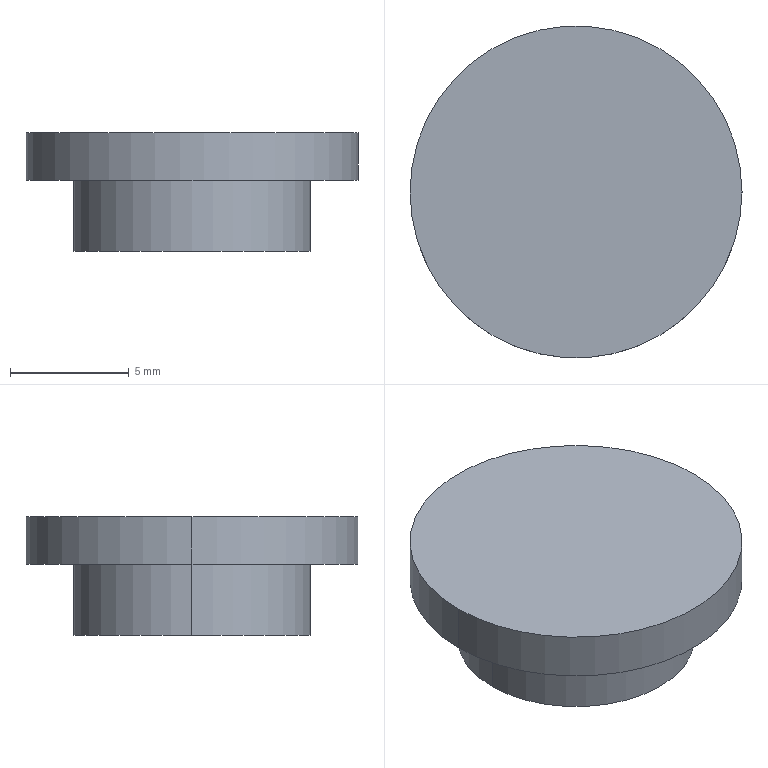Part | SolidWorks | features Extrusion 1, ICE 1 | 1 solid | 7 faces | box 14 x 14 x 5 mm | volume 543.496 mm3 | cylinder 4 | plane 3 | commonest cylinder face diameters 10 x2 14 x2
STEP:
#1=CARTESIAN_POINT('',(7.,0.,2.));
#2=VERTEX_POINT('',#1);
#3=CARTESIAN_POINT('',(-7.,0.,2.));
#4=VERTEX_POINT('',#3);
#5=CARTESIAN_POINT('',(0.,0.,2.));
#6=DIRECTION('',(0.,0.,1.));
#7=DIRECTION('',(1.,0.,0.));
#8=AXIS2_PLACEMENT_3D('',#5,#6,#7);
#9=CIRCLE('',#8,7.);
#10=EDGE_CURVE('',#2,#4,#9,.T.);
#11=ORIENTED_EDGE('',*,*,#10,.F.);
#12=CARTESIAN_POINT('',(7.,0.,0.));
#13=VERTEX_POINT('',#12);
#14=CARTESIAN_POINT('',(7.,0.,2.));
#15=DIRECTION('',(0.,0.,-1.));
#16=VECTOR('',#15,1000.);
#17=LINE('',#14,#16);
#18=EDGE_CURVE('',#2,#13,#17,.T.);
#19=ORIENTED_EDGE('',*,*,#18,.T.);
#20=CARTESIAN_POINT('',(-7.,0.,0.));
#21=VERTEX_POINT('',#20);
#22=CARTESIAN_POINT('',(0.,0.,0.));
#23=DIRECTION('',(0.,0.,1.));
#24=DIRECTION('',(1.,0.,0.));
#25=AXIS2_PLACEMENT_3D('',#22,#23,#24);
#26=CIRCLE('',#25,7.);
#27=EDGE_CURVE('',#13,#21,#26,.T.);
#28=ORIENTED_EDGE('',*,*,#27,.T.);
#29=CARTESIAN_POINT('',(-7.,0.,2.));
#30=DIRECTION('',(0.,0.,-1.));
#31=VECTOR('',#30,1000.);
#32=LINE('',#29,#31);
#33=EDGE_CURVE('',#4,#21,#32,.T.);
#34=ORIENTED_EDGE('',*,*,#33,.F.);
#35=EDGE_LOOP('',(#11,#19,#28,#34));
#36=FACE_OUTER_BOUND('',#35,.T.);
#37=CARTESIAN_POINT('',(0.,0.,2.));
#38=DIRECTION('',(0.,0.,-1.));
#39=DIRECTION('',(-1.,0.,0.));
#40=AXIS2_PLACEMENT_3D('',#37,#38,#39);
#41=CYLINDRICAL_SURFACE('',#40,7.);
#42=ADVANCED_FACE('',(#36),#41,.T.);
#43=CARTESIAN_POINT('',(5.,0.,-3.));
#44=VERTEX_POINT('',#43);
#45=CARTESIAN_POINT('',(-5.,0.,-3.));
#46=VERTEX_POINT('',#45);
#47=CARTESIAN_POINT('',(0.,0.,-3.));
#48=DIRECTION('',(0.,0.,1.));
#49=DIRECTION('',(1.,0.,0.));
#50=AXIS2_PLACEMENT_3D('',#47,#48,#49);
#51=CIRCLE('',#50,5.);
#52=EDGE_CURVE('',#44,#46,#51,.T.);
#53=ORIENTED_EDGE('',*,*,#52,.T.);
#54=CARTESIAN_POINT('',(-5.,0.,0.));
#55=VERTEX_POINT('',#54);
#56=CARTESIAN_POINT('',(-5.,0.,-3.));
#57=DIRECTION('',(0.,0.,1.));
#58=VECTOR('',#57,1000.);
#59=LINE('',#56,#58);
#60=EDGE_CURVE('',#46,#55,#59,.T.);
#61=ORIENTED_EDGE('',*,*,#60,.T.);
#62=CARTESIAN_POINT('',(5.,0.,0.));
#63=VERTEX_POINT('',#62);
#64=CARTESIAN_POINT('',(0.,0.,0.));
#65=DIRECTION('',(0.,0.,1.));
#66=DIRECTION('',(1.,0.,0.));
#67=AXIS2_PLACEMENT_3D('',#64,#65,#66);
#68=CIRCLE('',#67,5.);
#69=EDGE_CURVE('',#63,#55,#68,.T.);
#70=ORIENTED_EDGE('',*,*,#69,.F.);
#71=CARTESIAN_POINT('',(5.,0.,-3.));
#72=DIRECTION('',(0.,0.,1.));
#73=VECTOR('',#72,1000.);
#74=LINE('',#71,#73);
#75=EDGE_CURVE('',#44,#63,#74,.T.);
#76=ORIENTED_EDGE('',*,*,#75,.F.);
#77=EDGE_LOOP('',(#53,#61,#70,#76));
#78=FACE_OUTER_BOUND('',#77,.T.);
#79=CARTESIAN_POINT('',(0.,0.,-3.));
#80=DIRECTION('',(0.,0.,1.));
#81=DIRECTION('',(1.,0.,0.));
#82=AXIS2_PLACEMENT_3D('',#79,#80,#81);
#83=CYLINDRICAL_SURFACE('',#82,5.);
#84=ADVANCED_FACE('',(#78),#83,.T.);
#85=ORIENTED_EDGE('',*,*,#60,.F.);
#86=CARTESIAN_POINT('',(0.,0.,-3.));
#87=DIRECTION('',(0.,0.,1.));
#88=DIRECTION('',(1.,0.,0.));
#89=AXIS2_PLACEMENT_3D('',#86,#87,#88);
#90=CIRCLE('',#89,5.);
#91=EDGE_CURVE('',#46,#44,#90,.T.);
#92=ORIENTED_EDGE('',*,*,#91,.T.);
#93=ORIENTED_EDGE('',*,*,#75,.T.);
#94=CARTESIAN_POINT('',(0.,0.,0.));
#95=DIRECTION('',(0.,0.,1.));
#96=DIRECTION('',(1.,0.,0.));
#97=AXIS2_PLACEMENT_3D('',#94,#95,#96);
#98=CIRCLE('',#97,5.);
#99=EDGE_CURVE('',#55,#63,#98,.T.);
#100=ORIENTED_EDGE('',*,*,#99,.F.);
#101=EDGE_LOOP('',(#85,#92,#93,#100));
#102=FACE_OUTER_BOUND('',#101,.T.);
#103=CARTESIAN_POINT('',(0.,0.,-3.));
#104=DIRECTION('',(0.,0.,1.));
#105=DIRECTION('',(1.,0.,0.));
#106=AXIS2_PLACEMENT_3D('',#103,#104,#105);
#107=CYLINDRICAL_SURFACE('',#106,5.);
#108=ADVANCED_FACE('',(#102),#107,.T.);
#109=ORIENTED_EDGE('',*,*,#52,.F.);
#110=ORIENTED_EDGE('',*,*,#91,.F.);
#111=EDGE_LOOP('',(#109,#110));
#112=FACE_OUTER_BOUND('',#111,.T.);
#113=CARTESIAN_POINT('',(0.,0.,-3.));
#114=DIRECTION('',(0.,0.,1.));
#115=DIRECTION('',(1.,0.,0.));
#116=AXIS2_PLACEMENT_3D('',#113,#114,#115);
#117=PLANE('',#116);
#118=ADVANCED_FACE('',(#112),#117,.F.);
#119=ORIENTED_EDGE('',*,*,#18,.F.);
#120=CARTESIAN_POINT('',(0.,0.,2.));
#121=DIRECTION('',(0.,0.,1.));
#122=DIRECTION('',(1.,0.,0.));
#123=AXIS2_PLACEMENT_3D('',#120,#121,#122);
#124=CIRCLE('',#123,7.);
#125=EDGE_CURVE('',#4,#2,#124,.T.);
#126=ORIENTED_EDGE('',*,*,#125,.F.);
#127=ORIENTED_EDGE('',*,*,#33,.T.);
#128=CARTESIAN_POINT('',(0.,0.,0.));
#129=DIRECTION('',(0.,0.,1.));
#130=DIRECTION('',(1.,0.,0.));
#131=AXIS2_PLACEMENT_3D('',#128,#129,#130);
#132=CIRCLE('',#131,7.);
#133=EDGE_CURVE('',#21,#13,#132,.T.);
#134=ORIENTED_EDGE('',*,*,#133,.T.);
#135=EDGE_LOOP('',(#119,#126,#127,#134));
#136=FACE_OUTER_BOUND('',#135,.T.);
#137=CARTESIAN_POINT('',(0.,0.,2.));
#138=DIRECTION('',(0.,0.,-1.));
#139=DIRECTION('',(-1.,0.,0.));
#140=AXIS2_PLACEMENT_3D('',#137,#138,#139);
#141=CYLINDRICAL_SURFACE('',#140,7.);
#142=ADVANCED_FACE('',(#136),#141,.T.);
#143=ORIENTED_EDGE('',*,*,#125,.T.);
#144=ORIENTED_EDGE('',*,*,#10,.T.);
#145=EDGE_LOOP('',(#143,#144));
#146=FACE_OUTER_BOUND('',#145,.T.);
#147=CARTESIAN_POINT('',(0.,0.,2.));
#148=DIRECTION('',(0.,0.,1.));
#149=DIRECTION('',(1.,0.,0.));
#150=AXIS2_PLACEMENT_3D('',#147,#148,#149);
#151=PLANE('',#150);
#152=ADVANCED_FACE('',(#146),#151,.T.);
#153=ORIENTED_EDGE('',*,*,#69,.T.);
#154=ORIENTED_EDGE('',*,*,#99,.T.);
#155=EDGE_LOOP('',(#153,#154));
#156=FACE_BOUND('',#155,.T.);
#157=ORIENTED_EDGE('',*,*,#133,.F.);
#158=ORIENTED_EDGE('',*,*,#27,.F.);
#159=EDGE_LOOP('',(#157,#158));
#160=FACE_OUTER_BOUND('',#159,.T.);
#161=CARTESIAN_POINT('',(0.,0.,0.));
#162=DIRECTION('',(0.,0.,1.));
#163=DIRECTION('',(1.,0.,0.));
#164=AXIS2_PLACEMENT_3D('',#161,#162,#163);
#165=PLANE('',#164);
#166=ADVANCED_FACE('',(#156,#160),#165,.F.);
#167=CLOSED_SHELL('',(#42,#84,#108,#118,#142,#152,#166));
#168=MANIFOLD_SOLID_BREP('',#167);
#169=CARTESIAN_POINT('',(0.,0.,0.));
#170=DIRECTION('',(0.,0.,1.));
#171=DIRECTION('',(1.,0.,0.));
#172=AXIS2_PLACEMENT_3D('',#169,#170,#171);
#173=(LENGTH_UNIT()NAMED_UNIT(*)SI_UNIT(.MILLI.,.METRE.));
#174=UNCERTAINTY_MEASURE_WITH_UNIT(LENGTH_MEASURE(0.00001),#173,'','');
#175=(NAMED_UNIT(*)PLANE_ANGLE_UNIT()SI_UNIT($,.RADIAN.));
#176=(NAMED_UNIT(*)SI_UNIT($,.STERADIAN.)SOLID_ANGLE_UNIT());
#177=(GEOMETRIC_REPRESENTATION_CONTEXT(3)GLOBAL_UNCERTAINTY_ASSIGNED_CONTEXT((#174))GLOBAL_UNIT_ASSIGNED_CONTEXT((#173,#175,#176))REPRESENTATION_CONTEXT('',''));
#178=ADVANCED_BREP_SHAPE_REPRESENTATION('',(#168,#172),#177);